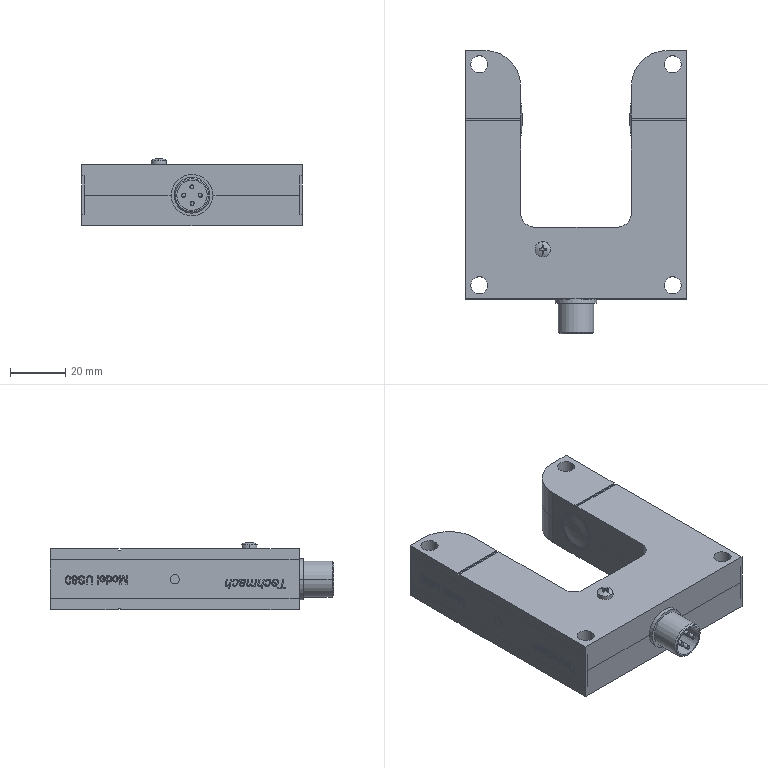Part | STEP file | US80aultrasonic sensor^Web-guide sensor assembly (take-up) | 14 solids | 951 faces | box 80.2 x 102.5 x 24.43 mm | volume 63293 mm3 | plane 437 | spline 284 | cylinder 166 | cone 50 | torus 8 | sphere 6 | commonest cylinder face diameters 2 x16 6.2 x16 3 x14 13 x14 1 x10 2.5 x10